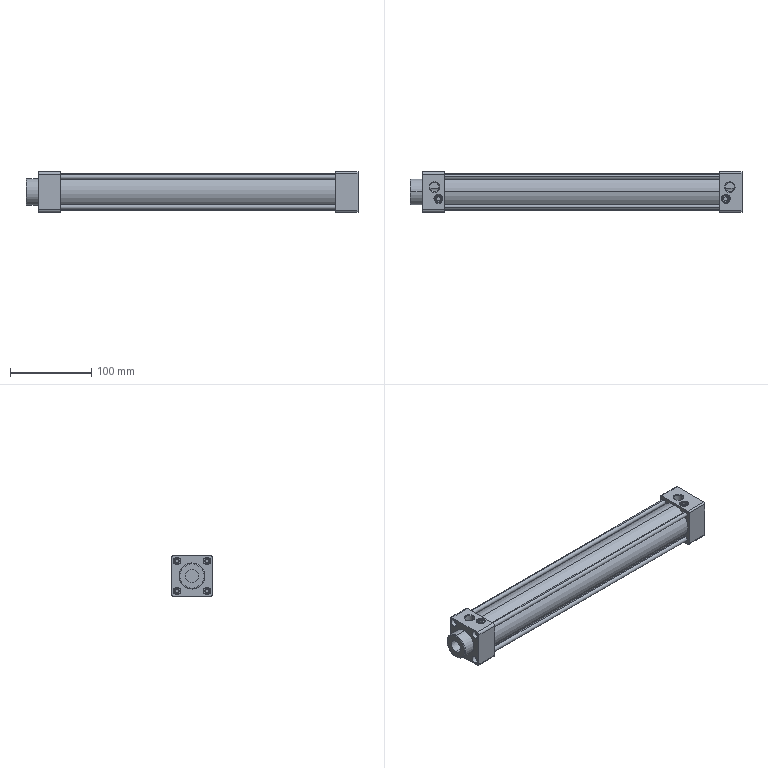Part | SolidWorks | features BaseBody 1 | 1 solid | 147 faces | box 408 x 50 x 50 mm | volume 287943 mm3 | cylinder 76 | plane 41 | cone 28 | torus 2 | commonest cylinder face diameters 4.917 x16 9.5 x16 6 x12 4 x4 5 x4 9.1 x4